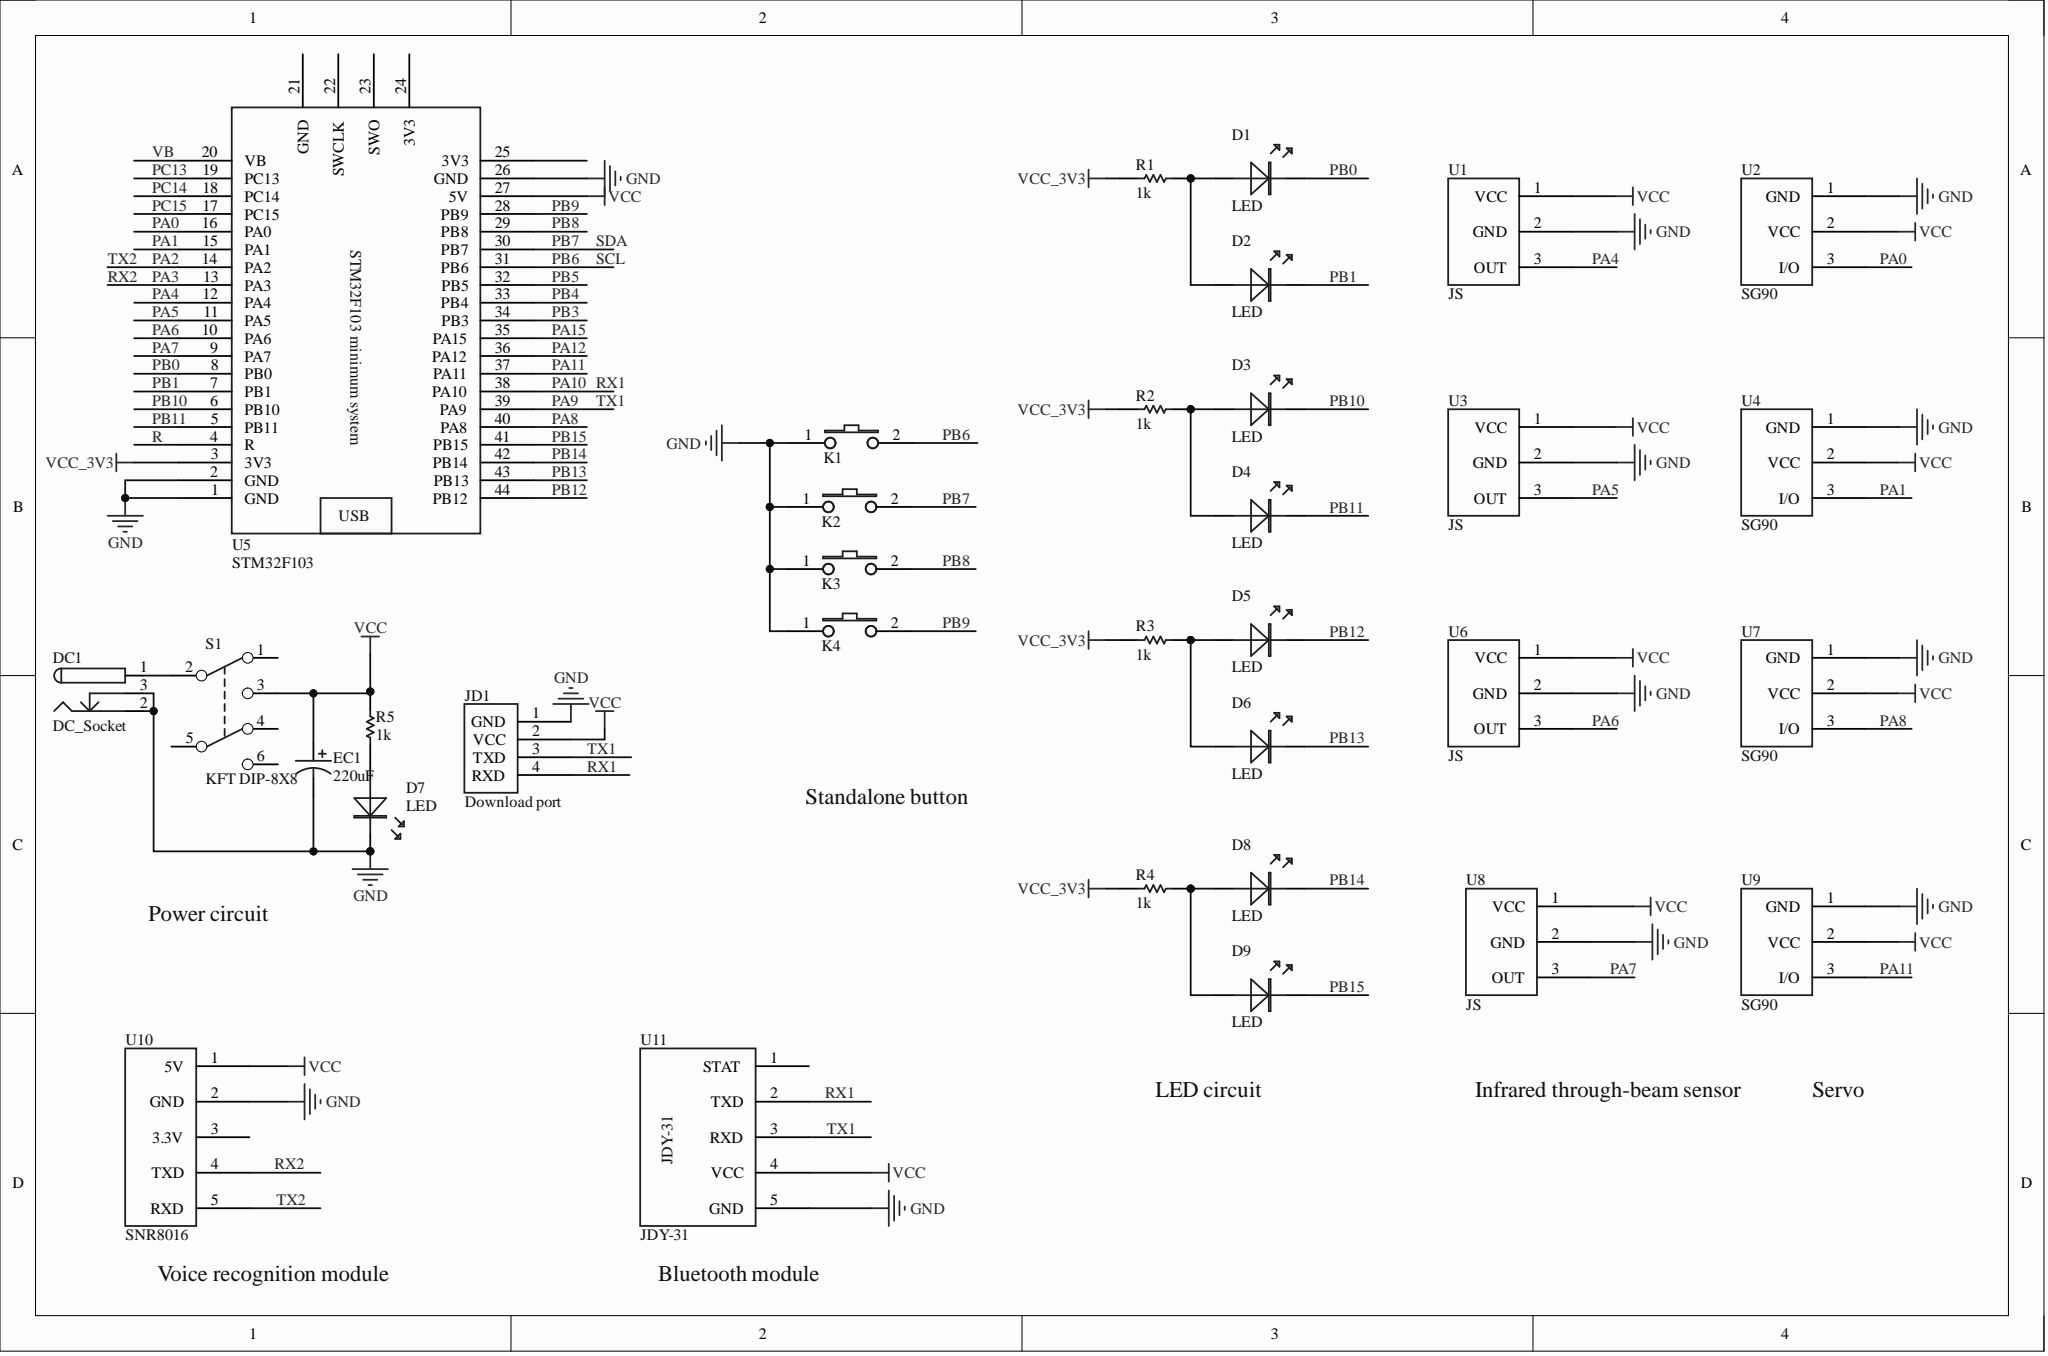Circuit board | Altium Designer | 33 parts | 33 nets
Bill of materials:
Comment,Description,Designator,Footprint,LibRef,Quantity
"LED","LED red, LED green","D1, D3, D5, D7, D8","LED5-GRE","LED","5"
"LED","LED red","D2, D4, D6, D9","LED5-RED","LED_1","4"
"DC_Socket","Power socket","DC1","DC-005","DC_Socket","1"
"220uF","Through-hole electrolytic capacitor","EC1","DIP-EC3.5X8X11.5","220uF","1"
"Download port","Download port","JD1","下载口","下载口_1","1"
"BUTTOM","Button","K1, K2, K3, K4","DIP-6X6X5","BUTTOM","4"
"1k","Resistor","R1, R2, R3, R4, R5","AXIAL0.3-1k","1k","5"
"KFT DIP-8X8","Self-locking button","S1","KFT DIP-8X8","KFT DIP-8X8_1","1"
"JS","Infrared through-beam sensor--counting","U1, U3, U6, U8","JS","JS_2","4"
"SG90","Servo","U2, U4, U7, U9","SG90","SG90_1","4"
"STM32F103","STM32F103","U5","STM32F103","STM32F103_1","1"
"SNR8016","Voice recognition module","U10","SNR8016","SNR8016_1","1"
"JDY-31","Bluetooth","U11","","JDY-31","1"
Netlist (Protel format):
[
D1
LED5-GRE
LED



]
[
D2
LED5-RED
LED



]
[
D3
LED5-GRE
LED



]
[
D4
LED5-RED
LED



]
[
D5
LED5-GRE
LED



]
[
D6
LED5-RED
LED



]
[
D7
LED5-GRE
LED



]
[
D8
LED5-GRE
LED



]
[
D9
LED5-RED
LED



]
[
DC1
DC-005
DC_Socket



]
[
EC1
DIP-EC3.5X8X11.5
220uF



]
[
JD1
下载口
Download port



]
[
K1
DIP-6X6X5
BUTTOM



]
[
K2
DIP-6X6X5
BUTTOM



]
[
K3
DIP-6X6X5
BUTTOM



]
[
K4
DIP-6X6X5
BUTTOM



]
[
R1
AXIAL0.3-1k
1k



]
[
R2
AXIAL0.3-1k
1k



]
[
R3
AXIAL0.3-1k
1k



]
[
R4
AXIAL0.3-1k
1k



]
[
R5
AXIAL0.3-1k
1k



]
[
S1
KFT DIP-8X8
KFT DIP-8X8



]
[
U1
JS
JS



]
[
U2
SG90
SG90



]
[
U3
JS
JS



]
[
U4
SG90
SG90



]
[
U5
STM32F103
STM32F103



]
[
U6
JS
JS



]
[
U7
SG90
SG90



]
[
U8
JS
JS



]
[
U9
SG90
SG90



]
[
U10
SNR8016
SNR8016



]
[
U11

JDY-31



]
(
VCC_3V3
R1-2
R2-2
R3-2
R4-2
U5-3
)
(
VCC
EC1-1
JD1-2
R5-2
S1-3
U1-1
U2-2
U3-1
U4-2
U5-27
U6-1
U7-2
U8-1
U9-2
U10-1
U11-4
)
(
PB15
D9-K
U5-41
)
(
PB14
D8-K
U5-42
)
(
PB13
D6-K
U5-43
)
(
PB12
D5-K
U5-44
)
(
PB11
D4-K
U5-5
)
(
PB10
D3-K
U5-6
)
(
PB9
K4-2
U5-28
)
(
PB8
K3-2
U5-29
)
(
PB7
K2-2
U5-30
)
(
PB6
K1-2
U5-31
)
(
PB1
D2-K
U5-7
)
(
PB0
D1-K
U5-8
)
(
PA11
U5-37
U9-3
)
(
PA10
JD1-4
U5-38
U11-2
)
(
PA9
JD1-3
U5-39
U11-3
)
(
PA8
U5-40
U7-3
)
(
PA7
U5-9
U8-3
)
(
PA6
U5-10
U6-3
)
(
PA5
U3-3
U5-11
)
(
PA4
U1-3
U5-12
)
(
PA3
U5-13
U10-4
)
(
PA2
U5-14
U10-5
)
(
PA1
U4-3
U5-15
)
(
PA0
U2-3
U5-16
)
(
NetDC1_1
DC1-1
S1-2
)
(
NetD8_A
D8-A
D9-A
R4-1
)
(
NetD7_A
D7-A
R5-1
)
(
NetD5_A
D5-A
D6-A
R3-1
)
(
NetD3_A
D3-A
D4-A
R2-1
)
(
NetD1_A
D1-A
D2-A
R1-1
)
(
GND
D7-K
DC1-2
DC1-3
EC1-2
JD1-1
K1-1
K2-1
K3-1
K4-1
U1-2
U2-1
U3-2
U4-1
U5-1
U5-2
U5-26
U6-2
U7-1
U8-2
U9-1
U10-2
U11-5
)